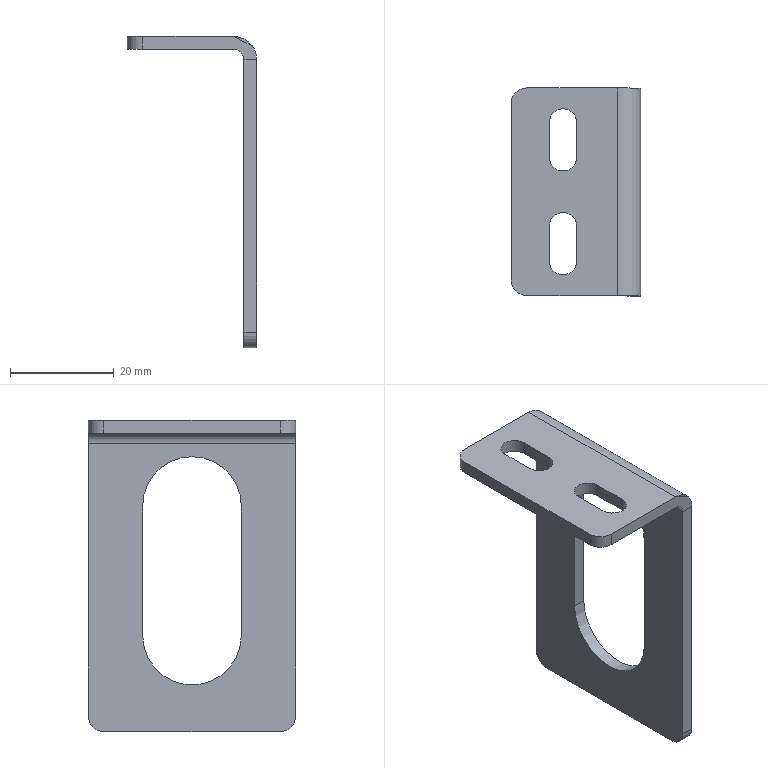Part | STEP file | 1 solid | 31 faces | box 25 x 40 x 60 mm | volume 5907 mm3 | plane 18 | cylinder 13 | commonest cylinder face diameters 5.3 x4 6 x4 19 x3 4 x1 9 x1